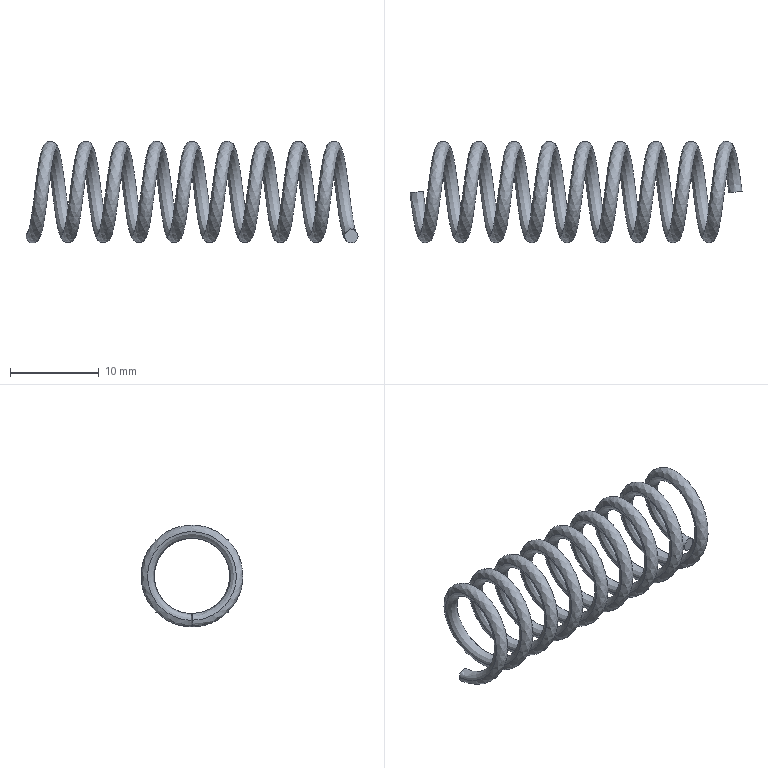Part | SolidWorks | features BaseBody 1 | 1 solid | 4 faces | box 37.488 x 11.5 x 11.5 mm | volume 503.734 mm3 | spline 2 | plane 2